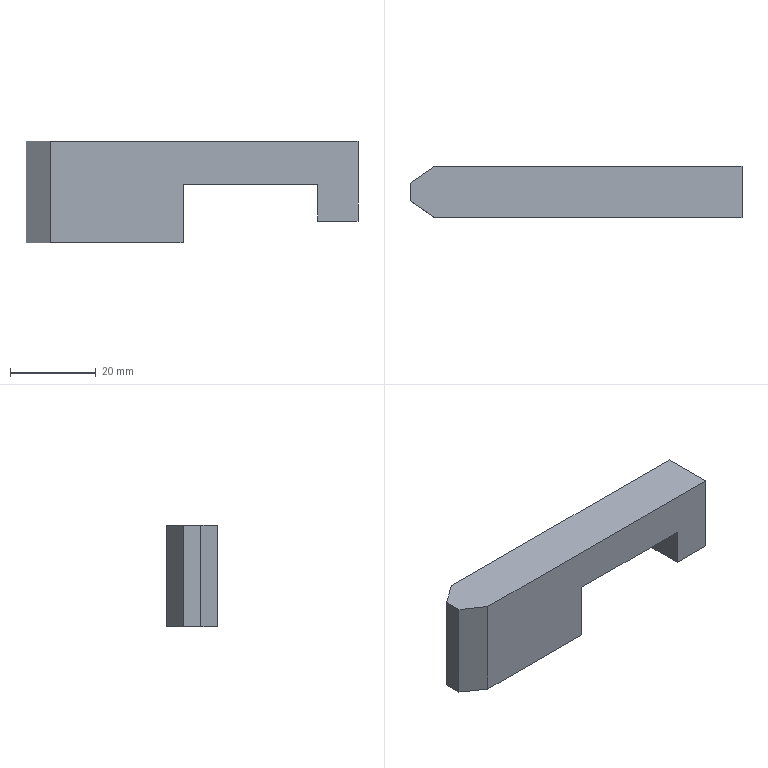Part | NX | features DIE-105 2 | 1 solid | 12 faces | box 77.6 x 12 x 23.626 mm | volume 15763 mm3 | plane 12
STEP:
#1=CARTESIAN_POINT('',(4355.038,-852.122,870.716));
#2=VERTEX_POINT('',#1);
#3=CARTESIAN_POINT('',(4355.038,-852.122,894.343));
#4=VERTEX_POINT('',#3);
#5=CARTESIAN_POINT('',(4355.038,-852.122,902.343));
#6=DIRECTION('',(0.000000002,0.,-1.));
#7=VECTOR('',#6,1000.);
#8=LINE('',#5,#7);
#9=EDGE_CURVE('',#2,#4,#8,.F.);
#10=ORIENTED_EDGE('',*,*,#9,.T.);
#11=CARTESIAN_POINT('',(4426.994,-852.122,894.343));
#12=VERTEX_POINT('',#11);
#13=CARTESIAN_POINT('',(4437.594,-852.122,894.343));
#14=DIRECTION('',(-1.,0.,0.));
#15=VECTOR('',#14,1000.);
#16=LINE('',#13,#15);
#17=EDGE_CURVE('',#12,#4,#16,.T.);
#18=ORIENTED_EDGE('',*,*,#17,.F.);
#19=CARTESIAN_POINT('',(4426.994,-852.122,875.716));
#20=VERTEX_POINT('',#19);
#21=CARTESIAN_POINT('',(4426.994,-852.122,902.343));
#22=DIRECTION('',(0.,0.,1.));
#23=VECTOR('',#22,1000.);
#24=LINE('',#21,#23);
#25=EDGE_CURVE('',#20,#12,#24,.T.);
#26=ORIENTED_EDGE('',*,*,#25,.F.);
#27=CARTESIAN_POINT('',(4417.594,-852.122,875.716));
#28=VERTEX_POINT('',#27);
#29=CARTESIAN_POINT('',(4023.354,-852.122,875.716));
#30=DIRECTION('',(-1.,0.,0.));
#31=VECTOR('',#30,1000.);
#32=LINE('',#29,#31);
#33=EDGE_CURVE('',#20,#28,#32,.T.);
#34=ORIENTED_EDGE('',*,*,#33,.T.);
#35=CARTESIAN_POINT('',(4417.594,-852.122,884.343));
#36=VERTEX_POINT('',#35);
#37=CARTESIAN_POINT('',(4417.594,-852.122,902.343));
#38=DIRECTION('',(0.,0.,1.));
#39=VECTOR('',#38,1000.);
#40=LINE('',#37,#39);
#41=EDGE_CURVE('',#28,#36,#40,.T.);
#42=ORIENTED_EDGE('',*,*,#41,.T.);
#43=CARTESIAN_POINT('',(4386.094,-852.122,884.343));
#44=VERTEX_POINT('',#43);
#45=CARTESIAN_POINT('',(4409.594,-852.122,884.343));
#46=DIRECTION('',(-1.,0.,0.));
#47=VECTOR('',#46,1000.);
#48=LINE('',#45,#47);
#49=EDGE_CURVE('',#36,#44,#48,.T.);
#50=ORIENTED_EDGE('',*,*,#49,.T.);
#51=CARTESIAN_POINT('',(4386.094,-852.122,870.716));
#52=VERTEX_POINT('',#51);
#53=CARTESIAN_POINT('',(4386.094,-852.122,902.343));
#54=DIRECTION('',(0.,0.,1.));
#55=VECTOR('',#54,1000.);
#56=LINE('',#53,#55);
#57=EDGE_CURVE('',#52,#44,#56,.T.);
#58=ORIENTED_EDGE('',*,*,#57,.F.);
#59=CARTESIAN_POINT('',(4437.594,-852.122,870.716));
#60=DIRECTION('',(1.,0.,0.));
#61=VECTOR('',#60,1000.);
#62=LINE('',#59,#61);
#63=EDGE_CURVE('',#2,#52,#62,.T.);
#64=ORIENTED_EDGE('',*,*,#63,.F.);
#65=EDGE_LOOP('',(#10,#18,#26,#34,#42,#50,#58,#64));
#66=FACE_BOUND('',#65,.T.);
#67=CARTESIAN_POINT('',(4437.594,-852.122,902.343));
#68=DIRECTION('',(0.,-1.,0.));
#69=DIRECTION('',(0.,0.,1.));
#70=AXIS2_PLACEMENT_3D('',#67,#68,#69);
#71=PLANE('',#70);
#72=ADVANCED_FACE('',(#66),#71,.F.);
#73=CARTESIAN_POINT('',(4386.094,-864.122,870.716));
#74=VERTEX_POINT('',#73);
#75=CARTESIAN_POINT('',(4386.094,-905.122,870.716));
#76=DIRECTION('',(0.,-1.,0.));
#77=VECTOR('',#76,1000.);
#78=LINE('',#75,#77);
#79=EDGE_CURVE('',#52,#74,#78,.T.);
#80=ORIENTED_EDGE('',*,*,#79,.F.);
#81=ORIENTED_EDGE('',*,*,#57,.T.);
#82=CARTESIAN_POINT('',(4386.094,-864.122,884.343));
#83=VERTEX_POINT('',#82);
#84=CARTESIAN_POINT('',(4386.094,-847.122,884.343));
#85=DIRECTION('',(0.,-1.,0.));
#86=VECTOR('',#85,1000.);
#87=LINE('',#84,#86);
#88=EDGE_CURVE('',#44,#83,#87,.T.);
#89=ORIENTED_EDGE('',*,*,#88,.T.);
#90=CARTESIAN_POINT('',(4386.094,-864.122,864.343));
#91=DIRECTION('',(0.,0.,1.));
#92=VECTOR('',#91,1000.);
#93=LINE('',#90,#92);
#94=EDGE_CURVE('',#74,#83,#93,.T.);
#95=ORIENTED_EDGE('',*,*,#94,.F.);
#96=EDGE_LOOP('',(#80,#81,#89,#95));
#97=FACE_BOUND('',#96,.T.);
#98=CARTESIAN_POINT('',(4386.094,-847.122,864.343));
#99=DIRECTION('',(1.,0.,0.));
#100=DIRECTION('',(0.,0.,1.));
#101=AXIS2_PLACEMENT_3D('',#98,#99,#100);
#102=PLANE('',#101);
#103=ADVANCED_FACE('',(#97),#102,.T.);
#104=CARTESIAN_POINT('',(4355.038,-864.122,870.716));
#105=VERTEX_POINT('',#104);
#106=CARTESIAN_POINT('',(4051.354,-864.122,870.716));
#107=DIRECTION('',(1.,0.,0.));
#108=VECTOR('',#107,1000.);
#109=LINE('',#106,#108);
#110=EDGE_CURVE('',#105,#74,#109,.T.);
#111=ORIENTED_EDGE('',*,*,#110,.F.);
#112=CARTESIAN_POINT('',(4349.394,-860.202,870.716));
#113=VERTEX_POINT('',#112);
#114=CARTESIAN_POINT('',(4169.396,-735.177,870.716));
#115=DIRECTION('',(-0.8213,0.5705,0.));
#116=VECTOR('',#115,1000.);
#117=LINE('',#114,#116);
#118=EDGE_CURVE('',#105,#113,#117,.T.);
#119=ORIENTED_EDGE('',*,*,#118,.T.);
#120=CARTESIAN_POINT('',(4349.394,-856.042,870.716));
#121=VERTEX_POINT('',#120);
#122=CARTESIAN_POINT('',(4349.394,-873.622,870.716));
#123=DIRECTION('',(0.,1.,0.));
#124=VECTOR('',#123,1000.);
#125=LINE('',#122,#124);
#126=EDGE_CURVE('',#113,#121,#125,.T.);
#127=ORIENTED_EDGE('',*,*,#126,.T.);
#128=CARTESIAN_POINT('',(4366.659,-844.05,870.716));
#129=DIRECTION('',(-0.8213,-0.5705,0.));
#130=VECTOR('',#129,1000.);
#131=LINE('',#128,#130);
#132=EDGE_CURVE('',#121,#2,#131,.F.);
#133=ORIENTED_EDGE('',*,*,#132,.T.);
#134=ORIENTED_EDGE('',*,*,#63,.T.);
#135=ORIENTED_EDGE('',*,*,#79,.T.);
#136=EDGE_LOOP('',(#111,#119,#127,#133,#134,#135));
#137=FACE_BOUND('',#136,.T.);
#138=CARTESIAN_POINT('',(4051.354,-905.122,870.716));
#139=DIRECTION('',(0.,0.,-1.));
#140=DIRECTION('',(-1.,0.,0.));
#141=AXIS2_PLACEMENT_3D('',#138,#139,#140);
#142=PLANE('',#141);
#143=ADVANCED_FACE('',(#137),#142,.T.);
#144=CARTESIAN_POINT('',(4417.594,-864.122,875.716));
#145=VERTEX_POINT('',#144);
#146=CARTESIAN_POINT('',(4417.594,-905.122,875.716));
#147=DIRECTION('',(0.,-1.,0.));
#148=VECTOR('',#147,1000.);
#149=LINE('',#146,#148);
#150=EDGE_CURVE('',#28,#145,#149,.T.);
#151=ORIENTED_EDGE('',*,*,#150,.F.);
#152=ORIENTED_EDGE('',*,*,#33,.F.);
#153=CARTESIAN_POINT('',(4426.994,-864.122,875.716));
#154=VERTEX_POINT('',#153);
#155=CARTESIAN_POINT('',(4426.994,-847.122,875.716));
#156=DIRECTION('',(0.,1.,0.));
#157=VECTOR('',#156,1000.);
#158=LINE('',#155,#157);
#159=EDGE_CURVE('',#154,#20,#158,.T.);
#160=ORIENTED_EDGE('',*,*,#159,.F.);
#161=CARTESIAN_POINT('',(4409.594,-864.122,875.716));
#162=DIRECTION('',(-1.,0.,0.));
#163=VECTOR('',#162,1000.);
#164=LINE('',#161,#163);
#165=EDGE_CURVE('',#154,#145,#164,.T.);
#166=ORIENTED_EDGE('',*,*,#165,.T.);
#167=EDGE_LOOP('',(#151,#152,#160,#166));
#168=FACE_BOUND('',#167,.T.);
#169=CARTESIAN_POINT('',(4023.354,-905.122,875.716));
#170=DIRECTION('',(0.,0.,-1.));
#171=DIRECTION('',(-1.,0.,0.));
#172=AXIS2_PLACEMENT_3D('',#169,#170,#171);
#173=PLANE('',#172);
#174=ADVANCED_FACE('',(#168),#173,.T.);
#175=ORIENTED_EDGE('',*,*,#159,.T.);
#176=ORIENTED_EDGE('',*,*,#25,.T.);
#177=CARTESIAN_POINT('',(4426.994,-864.122,894.343));
#178=VERTEX_POINT('',#177);
#179=CARTESIAN_POINT('',(4426.994,-847.122,894.343));
#180=DIRECTION('',(0.,-1.,0.));
#181=VECTOR('',#180,1000.);
#182=LINE('',#179,#181);
#183=EDGE_CURVE('',#12,#178,#182,.T.);
#184=ORIENTED_EDGE('',*,*,#183,.T.);
#185=CARTESIAN_POINT('',(4426.994,-864.122,864.343));
#186=DIRECTION('',(0.,0.,1.));
#187=VECTOR('',#186,1000.);
#188=LINE('',#185,#187);
#189=EDGE_CURVE('',#154,#178,#188,.T.);
#190=ORIENTED_EDGE('',*,*,#189,.F.);
#191=EDGE_LOOP('',(#175,#176,#184,#190));
#192=FACE_BOUND('',#191,.T.);
#193=CARTESIAN_POINT('',(4426.994,-847.122,864.343));
#194=DIRECTION('',(1.,0.,0.));
#195=DIRECTION('',(0.,0.,1.));
#196=AXIS2_PLACEMENT_3D('',#193,#194,#195);
#197=PLANE('',#196);
#198=ADVANCED_FACE('',(#192),#197,.T.);
#199=ORIENTED_EDGE('',*,*,#150,.T.);
#200=CARTESIAN_POINT('',(4417.594,-864.122,884.343));
#201=VERTEX_POINT('',#200);
#202=CARTESIAN_POINT('',(4417.594,-864.122,877.343));
#203=DIRECTION('',(0.,0.,1.));
#204=VECTOR('',#203,1000.);
#205=LINE('',#202,#204);
#206=EDGE_CURVE('',#145,#201,#205,.T.);
#207=ORIENTED_EDGE('',*,*,#206,.T.);
#208=CARTESIAN_POINT('',(4417.594,-858.122,884.343));
#209=DIRECTION('',(0.,1.,0.));
#210=VECTOR('',#209,1000.);
#211=LINE('',#208,#210);
#212=EDGE_CURVE('',#201,#36,#211,.T.);
#213=ORIENTED_EDGE('',*,*,#212,.T.);
#214=ORIENTED_EDGE('',*,*,#41,.F.);
#215=EDGE_LOOP('',(#199,#207,#213,#214));
#216=FACE_BOUND('',#215,.T.);
#217=CARTESIAN_POINT('',(4417.594,-858.122,877.343));
#218=DIRECTION('',(1.,0.,0.));
#219=DIRECTION('',(0.,0.,1.));
#220=AXIS2_PLACEMENT_3D('',#217,#218,#219);
#221=PLANE('',#220);
#222=ADVANCED_FACE('',(#216),#221,.F.);
#223=ORIENTED_EDGE('',*,*,#212,.F.);
#224=CARTESIAN_POINT('',(4351.094,-864.122,884.343));
#225=DIRECTION('',(-1.,0.,0.));
#226=VECTOR('',#225,1000.);
#227=LINE('',#224,#226);
#228=EDGE_CURVE('',#201,#83,#227,.T.);
#229=ORIENTED_EDGE('',*,*,#228,.T.);
#230=ORIENTED_EDGE('',*,*,#88,.F.);
#231=ORIENTED_EDGE('',*,*,#49,.F.);
#232=EDGE_LOOP('',(#223,#229,#230,#231));
#233=FACE_BOUND('',#232,.T.);
#234=CARTESIAN_POINT('',(4351.094,-858.122,884.343));
#235=DIRECTION('',(0.,0.,1.));
#236=DIRECTION('',(0.,-1.,0.));
#237=AXIS2_PLACEMENT_3D('',#234,#235,#236);
#238=PLANE('',#237);
#239=ADVANCED_FACE('',(#233),#238,.F.);
#240=ORIENTED_EDGE('',*,*,#17,.T.);
#241=CARTESIAN_POINT('',(4349.394,-856.042,894.343));
#242=VERTEX_POINT('',#241);
#243=CARTESIAN_POINT('',(4397.554,-822.59,894.343));
#244=DIRECTION('',(-0.8213,-0.5705,0.));
#245=VECTOR('',#244,1000.);
#246=LINE('',#243,#245);
#247=EDGE_CURVE('',#242,#4,#246,.F.);
#248=ORIENTED_EDGE('',*,*,#247,.F.);
#249=CARTESIAN_POINT('',(4349.394,-860.202,894.343));
#250=VERTEX_POINT('',#249);
#251=CARTESIAN_POINT('',(4349.394,-847.122,894.343));
#252=DIRECTION('',(0.,1.,0.));
#253=VECTOR('',#252,1000.);
#254=LINE('',#251,#253);
#255=EDGE_CURVE('',#250,#242,#254,.T.);
#256=ORIENTED_EDGE('',*,*,#255,.F.);
#257=CARTESIAN_POINT('',(4355.038,-864.122,894.343));
#258=VERTEX_POINT('',#257);
#259=CARTESIAN_POINT('',(4387.246,-886.494,894.343));
#260=DIRECTION('',(0.8213,-0.5705,0.));
#261=VECTOR('',#260,1000.);
#262=LINE('',#259,#261);
#263=EDGE_CURVE('',#258,#250,#262,.F.);
#264=ORIENTED_EDGE('',*,*,#263,.F.);
#265=CARTESIAN_POINT('',(4414.594,-864.122,894.343));
#266=DIRECTION('',(-1.,0.,0.));
#267=VECTOR('',#266,1000.);
#268=LINE('',#265,#267);
#269=EDGE_CURVE('',#178,#258,#268,.T.);
#270=ORIENTED_EDGE('',*,*,#269,.F.);
#271=ORIENTED_EDGE('',*,*,#183,.F.);
#272=EDGE_LOOP('',(#240,#248,#256,#264,#270,#271));
#273=FACE_BOUND('',#272,.T.);
#274=CARTESIAN_POINT('',(4414.594,-847.122,894.343));
#275=DIRECTION('',(0.,0.,1.));
#276=DIRECTION('',(0.,1.,0.));
#277=AXIS2_PLACEMENT_3D('',#274,#275,#276);
#278=PLANE('',#277);
#279=ADVANCED_FACE('',(#273),#278,.T.);
#280=ORIENTED_EDGE('',*,*,#126,.F.);
#281=CARTESIAN_POINT('',(4349.394,-860.202,-840.716));
#282=DIRECTION('',(0.,-0.000000001,1.));
#283=VECTOR('',#282,1000.);
#284=LINE('',#281,#283);
#285=EDGE_CURVE('',#113,#250,#284,.T.);
#286=ORIENTED_EDGE('',*,*,#285,.T.);
#287=ORIENTED_EDGE('',*,*,#255,.T.);
#288=CARTESIAN_POINT('',(4349.394,-856.042,882.843));
#289=DIRECTION('',(0.,0.000000001,1.));
#290=VECTOR('',#289,1000.);
#291=LINE('',#288,#290);
#292=EDGE_CURVE('',#242,#121,#291,.F.);
#293=ORIENTED_EDGE('',*,*,#292,.T.);
#294=EDGE_LOOP('',(#280,#286,#287,#293));
#295=FACE_BOUND('',#294,.T.);
#296=CARTESIAN_POINT('',(4349.394,-873.622,882.843));
#297=DIRECTION('',(1.,0.,0.));
#298=DIRECTION('',(0.,0.,1.));
#299=AXIS2_PLACEMENT_3D('',#296,#297,#298);
#300=PLANE('',#299);
#301=ADVANCED_FACE('',(#295),#300,.F.);
#302=ORIENTED_EDGE('',*,*,#269,.T.);
#303=CARTESIAN_POINT('',(4355.038,-864.122,-840.716));
#304=DIRECTION('',(0.000000002,0.,-1.));
#305=VECTOR('',#304,1000.);
#306=LINE('',#303,#305);
#307=EDGE_CURVE('',#258,#105,#306,.T.);
#308=ORIENTED_EDGE('',*,*,#307,.T.);
#309=ORIENTED_EDGE('',*,*,#110,.T.);
#310=ORIENTED_EDGE('',*,*,#94,.T.);
#311=ORIENTED_EDGE('',*,*,#228,.F.);
#312=ORIENTED_EDGE('',*,*,#206,.F.);
#313=ORIENTED_EDGE('',*,*,#165,.F.);
#314=ORIENTED_EDGE('',*,*,#189,.T.);
#315=EDGE_LOOP('',(#302,#308,#309,#310,#311,#312,#313,#314));
#316=FACE_BOUND('',#315,.T.);
#317=CARTESIAN_POINT('',(4437.594,-864.122,902.343));
#318=DIRECTION('',(0.,1.,0.));
#319=DIRECTION('',(0.,0.,1.));
#320=AXIS2_PLACEMENT_3D('',#317,#318,#319);
#321=PLANE('',#320);
#322=ADVANCED_FACE('',(#316),#321,.F.);
#323=ORIENTED_EDGE('',*,*,#247,.T.);
#324=ORIENTED_EDGE('',*,*,#9,.F.);
#325=ORIENTED_EDGE('',*,*,#132,.F.);
#326=ORIENTED_EDGE('',*,*,#292,.F.);
#327=EDGE_LOOP('',(#323,#324,#325,#326));
#328=FACE_BOUND('',#327,.T.);
#329=CARTESIAN_POINT('',(4366.659,-844.05,-840.716));
#330=DIRECTION('',(-0.5705,0.8213,-0.000000001));
#331=DIRECTION('',(-0.8213,-0.5705,0.));
#332=AXIS2_PLACEMENT_3D('',#329,#330,#331);
#333=PLANE('',#332);
#334=ADVANCED_FACE('',(#328),#333,.T.);
#335=ORIENTED_EDGE('',*,*,#263,.T.);
#336=ORIENTED_EDGE('',*,*,#285,.F.);
#337=ORIENTED_EDGE('',*,*,#118,.F.);
#338=ORIENTED_EDGE('',*,*,#307,.F.);
#339=EDGE_LOOP('',(#335,#336,#337,#338));
#340=FACE_BOUND('',#339,.T.);
#341=CARTESIAN_POINT('',(4366.659,-872.194,-840.716));
#342=DIRECTION('',(-0.5705,-0.8213,-0.000000001));
#343=DIRECTION('',(-0.8213,0.5705,0.));
#344=AXIS2_PLACEMENT_3D('',#341,#342,#343);
#345=PLANE('',#344);
#346=ADVANCED_FACE('',(#340),#345,.T.);
#347=CLOSED_SHELL('',(#72,#103,#143,#174,#198,#222,#239,#279,#301,#322,#334,#346));
#348=MANIFOLD_SOLID_BREP('',#347);
#349=(LENGTH_UNIT()NAMED_UNIT(*)SI_UNIT(.MILLI.,.METRE.));
#350=UNCERTAINTY_MEASURE_WITH_UNIT(LENGTH_MEASURE(0.00001),#349,'','');
#351=(NAMED_UNIT(*)PLANE_ANGLE_UNIT()SI_UNIT($,.RADIAN.));
#352=(NAMED_UNIT(*)SI_UNIT($,.STERADIAN.)SOLID_ANGLE_UNIT());
#353=(GEOMETRIC_REPRESENTATION_CONTEXT(3)GLOBAL_UNCERTAINTY_ASSIGNED_CONTEXT((#350))GLOBAL_UNIT_ASSIGNED_CONTEXT((#349,#351,#352))REPRESENTATION_CONTEXT('',''));
#354=ADVANCED_BREP_SHAPE_REPRESENTATION('',(#348),#353);